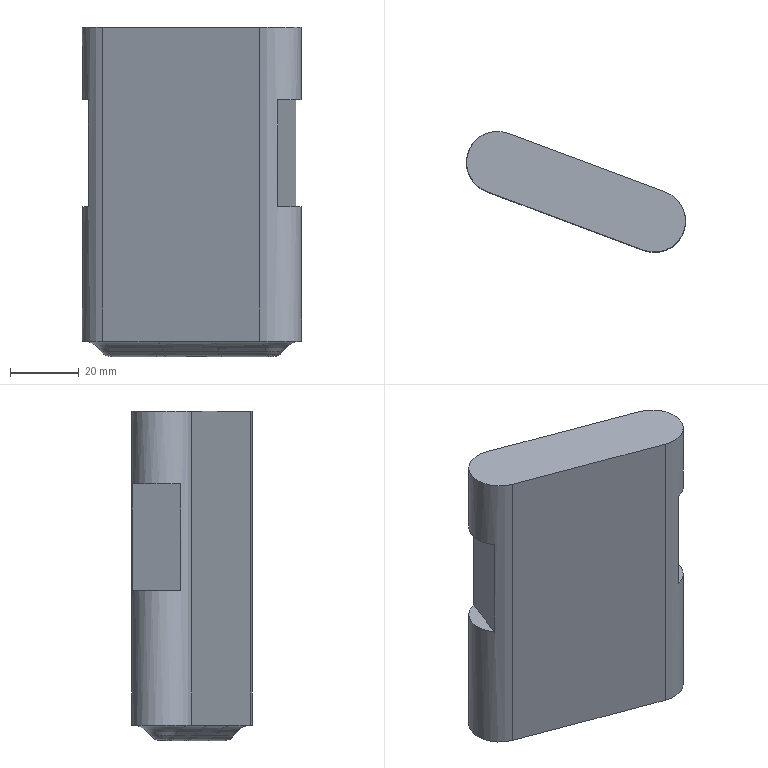Part | NX | features 8 2 | 1 solid | 31 faces | box 63.572 x 35.039 x 95.5 mm | volume 102490 mm3 | plane 11 | cylinder 10 | spline 8 | torus 2 | commonest cylinder face diameters 6 x4 13 x4 18 x2
STEP:
#1=CARTESIAN_POINT('',(108.541,59.531,91.));
#2=VERTEX_POINT('',#1);
#3=CARTESIAN_POINT('',(114.844,76.391,91.));
#4=VERTEX_POINT('',#3);
#5=CARTESIAN_POINT('',(111.693,67.961,91.));
#6=DIRECTION('',(0.,0.,-1.));
#7=DIRECTION('',(1.,0.,0.));
#8=AXIS2_PLACEMENT_3D('',#5,#6,#7);
#9=CIRCLE('',#8,9.);
#10=EDGE_CURVE('',#2,#4,#9,.T.);
#11=ORIENTED_EDGE('',*,*,#10,.F.);
#12=CARTESIAN_POINT('',(154.113,42.492,91.));
#13=VERTEX_POINT('',#12);
#14=CARTESIAN_POINT('',(154.113,42.492,91.));
#15=DIRECTION('',(0.9367,-0.3502,0.));
#16=VECTOR('',#15,1000.);
#17=LINE('',#14,#16);
#18=EDGE_CURVE('',#2,#13,#17,.T.);
#19=ORIENTED_EDGE('',*,*,#18,.T.);
#20=CARTESIAN_POINT('',(160.417,59.352,91.));
#21=VERTEX_POINT('',#20);
#22=CARTESIAN_POINT('',(157.265,50.922,91.));
#23=DIRECTION('',(0.,0.,-1.));
#24=DIRECTION('',(1.,0.,0.));
#25=AXIS2_PLACEMENT_3D('',#22,#23,#24);
#26=CIRCLE('',#25,9.);
#27=EDGE_CURVE('',#21,#13,#26,.T.);
#28=ORIENTED_EDGE('',*,*,#27,.F.);
#29=CARTESIAN_POINT('',(160.417,59.352,91.));
#30=DIRECTION('',(-0.9367,0.3502,0.));
#31=VECTOR('',#30,1000.);
#32=LINE('',#29,#31);
#33=EDGE_CURVE('',#21,#4,#32,.T.);
#34=ORIENTED_EDGE('',*,*,#33,.T.);
#35=EDGE_LOOP('',(#11,#19,#28,#34));
#36=FACE_BOUND('',#35,.T.);
#37=CARTESIAN_POINT('',(1075.,0.,91.));
#38=DIRECTION('',(0.,0.,1.));
#39=DIRECTION('',(-1.,0.,0.));
#40=AXIS2_PLACEMENT_3D('',#37,#38,#39);
#41=PLANE('',#40);
#42=ADVANCED_FACE('',(#36),#41,.T.);
#43=ORIENTED_EDGE('',*,*,#33,.F.);
#44=CARTESIAN_POINT('',(160.417,59.352,-0.0004651));
#45=VERTEX_POINT('',#44);
#46=CARTESIAN_POINT('',(160.417,59.352,-100.));
#47=DIRECTION('',(0.,0.,-1.));
#48=VECTOR('',#47,1000.);
#49=LINE('',#46,#48);
#50=EDGE_CURVE('',#21,#45,#49,.T.);
#51=ORIENTED_EDGE('',*,*,#50,.T.);
#52=CARTESIAN_POINT('',(146.714,64.517,-0.0002356));
#53=VERTEX_POINT('',#52);
#54=CARTESIAN_POINT('',(160.417,59.352,-0.0004651));
#55=CARTESIAN_POINT('',(156.358,60.87,-0.0004651));
#56=CARTESIAN_POINT('',(152.299,62.387,-0.0004651));
#57=CARTESIAN_POINT('',(147.727,64.097,-0.0004651));
#58=CARTESIAN_POINT('',(147.214,64.289,-0.0004651));
#59=CARTESIAN_POINT('',(146.7,64.48,-0.0004651));
#60=B_SPLINE_CURVE_WITH_KNOTS('',3,(#54,#55,#56,#57,#58,#59),.UNSPECIFIED.,.F.,.F.,(4,2,4),(0.,0.8877,1.),.UNSPECIFIED.);
#61=EDGE_CURVE('',#45,#53,#60,.T.);
#62=ORIENTED_EDGE('',*,*,#61,.T.);
#63=CARTESIAN_POINT('',(130.403,70.602,-0.0003097));
#64=VERTEX_POINT('',#63);
#65=CARTESIAN_POINT('',(130.393,70.577,-0.0004711));
#66=CARTESIAN_POINT('',(135.829,68.545,-0.0004711));
#67=CARTESIAN_POINT('',(141.265,66.513,-0.0004711));
#68=CARTESIAN_POINT('',(146.7,64.48,-0.0004711));
#69=B_SPLINE_CURVE_WITH_KNOTS('',3,(#65,#66,#67,#68),.UNSPECIFIED.,.F.,.F.,(4,4),(0.,1.),.PIECEWISE_BEZIER_KNOTS.);
#70=EDGE_CURVE('',#64,#53,#69,.T.);
#71=ORIENTED_EDGE('',*,*,#70,.F.);
#72=CARTESIAN_POINT('',(114.844,76.391,-0.0004651));
#73=VERTEX_POINT('',#72);
#74=CARTESIAN_POINT('',(130.393,70.577,-0.0004651));
#75=CARTESIAN_POINT('',(126.432,72.058,-0.0004651));
#76=CARTESIAN_POINT('',(122.471,73.539,-0.0004651));
#77=CARTESIAN_POINT('',(117.288,75.477,-0.0004651));
#78=CARTESIAN_POINT('',(116.066,75.934,-0.0004651));
#79=CARTESIAN_POINT('',(114.844,76.391,-0.0004651));
#80=B_SPLINE_CURVE_WITH_KNOTS('',3,(#74,#75,#76,#77,#78,#79),.UNSPECIFIED.,.F.,.F.,(4,2,4),(0.,0.7642,1.),.UNSPECIFIED.);
#81=EDGE_CURVE('',#64,#73,#80,.T.);
#82=ORIENTED_EDGE('',*,*,#81,.T.);
#83=CARTESIAN_POINT('',(114.844,76.391,-100.));
#84=DIRECTION('',(0.,0.,1.));
#85=VECTOR('',#84,1000.);
#86=LINE('',#83,#85);
#87=EDGE_CURVE('',#73,#4,#86,.T.);
#88=ORIENTED_EDGE('',*,*,#87,.T.);
#89=EDGE_LOOP('',(#43,#51,#62,#71,#82,#88));
#90=FACE_BOUND('',#89,.T.);
#91=CARTESIAN_POINT('',(160.417,59.352,-100.));
#92=DIRECTION('',(-0.3502,-0.9367,0.));
#93=DIRECTION('',(0.9367,-0.3502,0.));
#94=AXIS2_PLACEMENT_3D('',#91,#92,#93);
#95=PLANE('',#94);
#96=ADVANCED_FACE('',(#90),#95,.F.);
#97=CARTESIAN_POINT('',(159.328,42.162,70.));
#98=VERTEX_POINT('',#97);
#99=CARTESIAN_POINT('',(164.569,56.181,70.));
#100=VERTEX_POINT('',#99);
#101=CARTESIAN_POINT('',(157.265,50.922,70.));
#102=DIRECTION('',(0.,0.,1.));
#103=DIRECTION('',(1.,0.,0.));
#104=AXIS2_PLACEMENT_3D('',#101,#102,#103);
#105=CIRCLE('',#104,9.);
#106=EDGE_CURVE('',#98,#100,#105,.T.);
#107=ORIENTED_EDGE('',*,*,#106,.T.);
#108=CARTESIAN_POINT('',(164.569,56.181,39.));
#109=VERTEX_POINT('',#108);
#110=CARTESIAN_POINT('',(164.569,56.181,-100.));
#111=DIRECTION('',(0.,0.,-1.));
#112=VECTOR('',#111,1000.);
#113=LINE('',#110,#112);
#114=EDGE_CURVE('',#100,#109,#113,.T.);
#115=ORIENTED_EDGE('',*,*,#114,.T.);
#116=CARTESIAN_POINT('',(159.328,42.162,39.));
#117=VERTEX_POINT('',#116);
#118=CARTESIAN_POINT('',(157.265,50.922,39.));
#119=DIRECTION('',(0.,0.,-1.));
#120=DIRECTION('',(-1.,0.,0.));
#121=AXIS2_PLACEMENT_3D('',#118,#119,#120);
#122=CIRCLE('',#121,9.);
#123=EDGE_CURVE('',#109,#117,#122,.T.);
#124=ORIENTED_EDGE('',*,*,#123,.T.);
#125=CARTESIAN_POINT('',(159.328,42.162,-100.));
#126=DIRECTION('',(0.,0.,1.));
#127=VECTOR('',#126,1000.);
#128=LINE('',#125,#127);
#129=EDGE_CURVE('',#117,#98,#128,.T.);
#130=ORIENTED_EDGE('',*,*,#129,.T.);
#131=EDGE_LOOP('',(#107,#115,#124,#130));
#132=FACE_BOUND('',#131,.T.);
#133=ORIENTED_EDGE('',*,*,#27,.T.);
#134=CARTESIAN_POINT('',(154.113,42.492,-0.000465));
#135=VERTEX_POINT('',#134);
#136=CARTESIAN_POINT('',(154.113,42.492,-100.));
#137=DIRECTION('',(0.,0.,1.));
#138=VECTOR('',#137,1000.);
#139=LINE('',#136,#138);
#140=EDGE_CURVE('',#135,#13,#139,.T.);
#141=ORIENTED_EDGE('',*,*,#140,.F.);
#142=CARTESIAN_POINT('',(157.265,50.922,-0.000465));
#143=DIRECTION('',(-0.000000001,0.000000001,1.));
#144=DIRECTION('',(0.,-1.,0.000000001));
#145=AXIS2_PLACEMENT_3D('',#142,#143,#144);
#146=CIRCLE('',#145,9.);
#147=EDGE_CURVE('',#45,#135,#146,.F.);
#148=ORIENTED_EDGE('',*,*,#147,.F.);
#149=ORIENTED_EDGE('',*,*,#50,.F.);
#150=EDGE_LOOP('',(#133,#141,#148,#149));
#151=FACE_BOUND('',#150,.T.);
#152=CARTESIAN_POINT('',(157.265,50.922,-100.));
#153=DIRECTION('',(0.,0.,1.));
#154=DIRECTION('',(-1.,0.,0.));
#155=AXIS2_PLACEMENT_3D('',#152,#153,#154);
#156=CYLINDRICAL_SURFACE('',#155,9.);
#157=ADVANCED_FACE('',(#132,#151),#156,.T.);
#158=CARTESIAN_POINT('',(104.389,62.702,39.));
#159=VERTEX_POINT('',#158);
#160=CARTESIAN_POINT('',(109.63,76.721,39.));
#161=VERTEX_POINT('',#160);
#162=CARTESIAN_POINT('',(111.693,67.961,39.));
#163=DIRECTION('',(0.,0.,-1.));
#164=DIRECTION('',(-1.,0.,0.));
#165=AXIS2_PLACEMENT_3D('',#162,#163,#164);
#166=CIRCLE('',#165,9.);
#167=EDGE_CURVE('',#159,#161,#166,.T.);
#168=ORIENTED_EDGE('',*,*,#167,.T.);
#169=CARTESIAN_POINT('',(109.63,76.721,70.));
#170=VERTEX_POINT('',#169);
#171=CARTESIAN_POINT('',(109.63,76.721,-100.));
#172=DIRECTION('',(0.,0.,1.));
#173=VECTOR('',#172,1000.);
#174=LINE('',#171,#173);
#175=EDGE_CURVE('',#161,#170,#174,.T.);
#176=ORIENTED_EDGE('',*,*,#175,.T.);
#177=CARTESIAN_POINT('',(104.389,62.702,70.));
#178=VERTEX_POINT('',#177);
#179=CARTESIAN_POINT('',(111.693,67.961,70.));
#180=DIRECTION('',(0.,0.,1.));
#181=DIRECTION('',(1.,0.,0.));
#182=AXIS2_PLACEMENT_3D('',#179,#180,#181);
#183=CIRCLE('',#182,9.);
#184=EDGE_CURVE('',#170,#178,#183,.T.);
#185=ORIENTED_EDGE('',*,*,#184,.T.);
#186=CARTESIAN_POINT('',(104.389,62.702,-100.));
#187=DIRECTION('',(0.,0.,-1.));
#188=VECTOR('',#187,1000.);
#189=LINE('',#186,#188);
#190=EDGE_CURVE('',#178,#159,#189,.T.);
#191=ORIENTED_EDGE('',*,*,#190,.T.);
#192=EDGE_LOOP('',(#168,#176,#185,#191));
#193=FACE_BOUND('',#192,.T.);
#194=ORIENTED_EDGE('',*,*,#87,.F.);
#195=CARTESIAN_POINT('',(108.541,59.531,-0.0004651));
#196=VERTEX_POINT('',#195);
#197=CARTESIAN_POINT('',(111.693,67.961,-0.0004651));
#198=DIRECTION('',(0.000000001,-0.000000001,-1.));
#199=DIRECTION('',(0.,1.,-0.000000001));
#200=AXIS2_PLACEMENT_3D('',#197,#198,#199);
#201=CIRCLE('',#200,9.);
#202=EDGE_CURVE('',#196,#73,#201,.T.);
#203=ORIENTED_EDGE('',*,*,#202,.F.);
#204=CARTESIAN_POINT('',(108.541,59.531,-100.));
#205=DIRECTION('',(0.,0.,-1.));
#206=VECTOR('',#205,1000.);
#207=LINE('',#204,#206);
#208=EDGE_CURVE('',#2,#196,#207,.T.);
#209=ORIENTED_EDGE('',*,*,#208,.F.);
#210=ORIENTED_EDGE('',*,*,#10,.T.);
#211=EDGE_LOOP('',(#194,#203,#209,#210));
#212=FACE_BOUND('',#211,.T.);
#213=CARTESIAN_POINT('',(111.693,67.961,-100.));
#214=DIRECTION('',(0.,0.,-1.));
#215=DIRECTION('',(1.,0.,0.));
#216=AXIS2_PLACEMENT_3D('',#213,#214,#215);
#217=CYLINDRICAL_SURFACE('',#216,9.);
#218=ADVANCED_FACE('',(#193,#212),#217,.T.);
#219=ORIENTED_EDGE('',*,*,#208,.T.);
#220=CARTESIAN_POINT('',(124.09,53.717,-0.0004681));
#221=VERTEX_POINT('',#220);
#222=CARTESIAN_POINT('',(108.541,59.531,-0.0004651));
#223=CARTESIAN_POINT('',(112.6,58.013,-0.0004651));
#224=CARTESIAN_POINT('',(116.658,56.496,-0.0004651));
#225=CARTESIAN_POINT('',(121.841,54.558,-0.0004651));
#226=CARTESIAN_POINT('',(122.966,54.137,-0.0004651));
#227=CARTESIAN_POINT('',(124.09,53.717,-0.0004651));
#228=B_SPLINE_CURVE_WITH_KNOTS('',3,(#222,#223,#224,#225,#226,#227),.UNSPECIFIED.,.F.,.F.,(4,2,4),(0.,0.7831,1.),.UNSPECIFIED.);
#229=EDGE_CURVE('',#196,#221,#228,.T.);
#230=ORIENTED_EDGE('',*,*,#229,.T.);
#231=CARTESIAN_POINT('',(140.397,47.62,-0.000468));
#232=VERTEX_POINT('',#231);
#233=CARTESIAN_POINT('',(140.397,47.62,-0.000471));
#234=CARTESIAN_POINT('',(134.961,49.653,-0.000471));
#235=CARTESIAN_POINT('',(129.525,51.685,-0.0004711));
#236=CARTESIAN_POINT('',(124.09,53.717,-0.0004711));
#237=B_SPLINE_CURVE_WITH_KNOTS('',3,(#233,#234,#235,#236),.UNSPECIFIED.,.F.,.F.,(4,4),(0.,1.),.PIECEWISE_BEZIER_KNOTS.);
#238=EDGE_CURVE('',#232,#221,#237,.T.);
#239=ORIENTED_EDGE('',*,*,#238,.F.);
#240=CARTESIAN_POINT('',(140.397,47.62,-0.0004651));
#241=CARTESIAN_POINT('',(144.445,46.107,-0.0004651));
#242=CARTESIAN_POINT('',(148.494,44.593,-0.000465));
#243=CARTESIAN_POINT('',(153.066,42.884,-0.000465));
#244=CARTESIAN_POINT('',(153.589,42.688,-0.000465));
#245=CARTESIAN_POINT('',(154.113,42.492,-0.000465));
#246=B_SPLINE_CURVE_WITH_KNOTS('',3,(#240,#241,#242,#243,#244,#245),.UNSPECIFIED.,.F.,.F.,(4,2,4),(0.,0.8855,1.),.UNSPECIFIED.);
#247=EDGE_CURVE('',#232,#135,#246,.T.);
#248=ORIENTED_EDGE('',*,*,#247,.T.);
#249=ORIENTED_EDGE('',*,*,#140,.T.);
#250=ORIENTED_EDGE('',*,*,#18,.F.);
#251=EDGE_LOOP('',(#219,#230,#239,#248,#249,#250));
#252=FACE_BOUND('',#251,.T.);
#253=CARTESIAN_POINT('',(154.113,42.492,-100.));
#254=DIRECTION('',(0.3502,0.9367,0.));
#255=DIRECTION('',(0.9367,-0.3502,0.));
#256=AXIS2_PLACEMENT_3D('',#253,#254,#255);
#257=PLANE('',#256);
#258=ADVANCED_FACE('',(#252),#257,.F.);
#259=CARTESIAN_POINT('',(143.899,56.987,-4.5));
#260=VERTEX_POINT('',#259);
#261=CARTESIAN_POINT('',(157.615,51.859,-4.5));
#262=VERTEX_POINT('',#261);
#263=CARTESIAN_POINT('',(150.757,54.423,-4.5));
#264=DIRECTION('',(0.9367,-0.3502,0.000000001));
#265=VECTOR('',#264,1000.);
#266=LINE('',#263,#265);
#267=EDGE_CURVE('',#260,#262,#266,.T.);
#268=ORIENTED_EDGE('',*,*,#267,.T.);
#269=CARTESIAN_POINT('',(156.915,49.985,-4.5));
#270=VERTEX_POINT('',#269);
#271=CARTESIAN_POINT('',(157.265,50.922,-4.5));
#272=DIRECTION('',(-0.000000001,0.000000001,1.));
#273=DIRECTION('',(-0.09584,-0.9954,0.000000001));
#274=AXIS2_PLACEMENT_3D('',#271,#272,#273);
#275=CIRCLE('',#274,1.);
#276=EDGE_CURVE('',#270,#262,#275,.T.);
#277=ORIENTED_EDGE('',*,*,#276,.F.);
#278=CARTESIAN_POINT('',(143.198,55.114,-4.5));
#279=VERTEX_POINT('',#278);
#280=CARTESIAN_POINT('',(150.057,52.55,-4.5));
#281=DIRECTION('',(0.9367,-0.3502,0.000000001));
#282=VECTOR('',#281,1000.);
#283=LINE('',#280,#282);
#284=EDGE_CURVE('',#279,#270,#283,.T.);
#285=ORIENTED_EDGE('',*,*,#284,.F.);
#286=CARTESIAN_POINT('',(126.891,61.211,-4.5));
#287=VERTEX_POINT('',#286);
#288=CARTESIAN_POINT('',(126.891,61.211,-4.5));
#289=CARTESIAN_POINT('',(132.327,59.178,-4.5));
#290=CARTESIAN_POINT('',(137.763,57.146,-4.5));
#291=CARTESIAN_POINT('',(143.198,55.114,-4.5));
#292=B_SPLINE_CURVE_WITH_KNOTS('',3,(#288,#289,#290,#291),.UNSPECIFIED.,.F.,.F.,(4,4),(0.,1.),.PIECEWISE_BEZIER_KNOTS.);
#293=EDGE_CURVE('',#287,#279,#292,.T.);
#294=ORIENTED_EDGE('',*,*,#293,.F.);
#295=CARTESIAN_POINT('',(124.472,62.115,-4.5));
#296=VERTEX_POINT('',#295);
#297=CARTESIAN_POINT('',(125.681,61.663,-4.5));
#298=DIRECTION('',(0.9367,-0.3502,0.000000001));
#299=VECTOR('',#298,1000.);
#300=LINE('',#297,#299);
#301=EDGE_CURVE('',#296,#287,#300,.T.);
#302=ORIENTED_EDGE('',*,*,#301,.F.);
#303=CARTESIAN_POINT('',(125.172,63.989,-4.5));
#304=VERTEX_POINT('',#303);
#305=CARTESIAN_POINT('',(125.172,63.989,-4.5));
#306=CARTESIAN_POINT('',(124.472,62.115,-4.5));
#307=B_SPLINE_CURVE_WITH_KNOTS('',1,(#305,#306),.UNSPECIFIED.,.F.,.F.,(2,2),(0.,1.),.PIECEWISE_BEZIER_KNOTS.);
#308=EDGE_CURVE('',#304,#296,#307,.T.);
#309=ORIENTED_EDGE('',*,*,#308,.F.);
#310=CARTESIAN_POINT('',(127.592,63.084,-4.5));
#311=VERTEX_POINT('',#310);
#312=CARTESIAN_POINT('',(126.382,63.536,-4.5));
#313=DIRECTION('',(-0.9367,0.3502,-0.000000001));
#314=VECTOR('',#313,1000.);
#315=LINE('',#312,#314);
#316=EDGE_CURVE('',#311,#304,#315,.T.);
#317=ORIENTED_EDGE('',*,*,#316,.F.);
#318=CARTESIAN_POINT('',(127.592,63.084,-4.5));
#319=CARTESIAN_POINT('',(133.027,61.052,-4.5));
#320=CARTESIAN_POINT('',(138.463,59.019,-4.5));
#321=CARTESIAN_POINT('',(143.899,56.987,-4.5));
#322=B_SPLINE_CURVE_WITH_KNOTS('',3,(#318,#319,#320,#321),.UNSPECIFIED.,.F.,.F.,(4,4),(0.,1.),.PIECEWISE_BEZIER_KNOTS.);
#323=EDGE_CURVE('',#311,#260,#322,.T.);
#324=ORIENTED_EDGE('',*,*,#323,.T.);
#325=EDGE_LOOP('',(#268,#277,#285,#294,#302,#309,#317,#324));
#326=FACE_BOUND('',#325,.T.);
#327=CARTESIAN_POINT('',(143.198,55.114,-4.5));
#328=DIRECTION('',(-0.000000001,0.000000001,1.));
#329=DIRECTION('',(-0.9367,0.3502,-0.000000001));
#330=AXIS2_PLACEMENT_3D('',#327,#328,#329);
#331=PLANE('',#330);
#332=ADVANCED_FACE('',(#326),#331,.F.);
#333=ORIENTED_EDGE('',*,*,#308,.T.);
#334=CARTESIAN_POINT('',(111.342,67.024,-4.5));
#335=VERTEX_POINT('',#334);
#336=CARTESIAN_POINT('',(111.342,67.024,-4.5));
#337=CARTESIAN_POINT('',(115.719,65.388,-4.5));
#338=CARTESIAN_POINT('',(120.095,63.751,-4.5));
#339=CARTESIAN_POINT('',(124.472,62.115,-4.5));
#340=B_SPLINE_CURVE_WITH_KNOTS('',3,(#336,#337,#338,#339),.UNSPECIFIED.,.F.,.F.,(4,4),(0.,1.),.PIECEWISE_BEZIER_KNOTS.);
#341=EDGE_CURVE('',#335,#296,#340,.T.);
#342=ORIENTED_EDGE('',*,*,#341,.F.);
#343=CARTESIAN_POINT('',(112.043,68.897,-4.5));
#344=VERTEX_POINT('',#343);
#345=CARTESIAN_POINT('',(112.043,68.897,-4.5));
#346=CARTESIAN_POINT('',(111.552,69.081,-4.5));
#347=CARTESIAN_POINT('',(110.939,68.801,-4.5));
#348=CARTESIAN_POINT('',(110.573,67.82,-4.5));
#349=CARTESIAN_POINT('',(110.852,67.207,-4.5));
#350=CARTESIAN_POINT('',(111.342,67.024,-4.5));
#351=B_SPLINE_CURVE_WITH_KNOTS('',3,(#345,#346,#347,#348,#349,#350),.UNSPECIFIED.,.F.,.F.,(4,2,4),(0.,0.5,1.),.UNSPECIFIED.);
#352=EDGE_CURVE('',#344,#335,#351,.T.);
#353=ORIENTED_EDGE('',*,*,#352,.F.);
#354=CARTESIAN_POINT('',(112.043,68.897,-4.5));
#355=CARTESIAN_POINT('',(125.172,63.989,-4.5));
#356=B_SPLINE_CURVE_WITH_KNOTS('',1,(#354,#355),.UNSPECIFIED.,.F.,.F.,(2,2),(0.,1.),.PIECEWISE_BEZIER_KNOTS.);
#357=EDGE_CURVE('',#344,#304,#356,.T.);
#358=ORIENTED_EDGE('',*,*,#357,.T.);
#359=EDGE_LOOP('',(#333,#342,#353,#358));
#360=FACE_BOUND('',#359,.T.);
#361=CARTESIAN_POINT('',(126.891,61.211,-4.5));
#362=DIRECTION('',(0.000000001,-0.000000001,-1.));
#363=DIRECTION('',(0.9367,-0.3502,0.000000001));
#364=AXIS2_PLACEMENT_3D('',#361,#362,#363);
#365=PLANE('',#364);
#366=ADVANCED_FACE('',(#360),#365,.T.);
#367=CARTESIAN_POINT('',(126.065,66.378,-3.079));
#368=VERTEX_POINT('',#367);
#369=CARTESIAN_POINT('',(128.485,65.473,-3.079));
#370=VERTEX_POINT('',#369);
#371=CARTESIAN_POINT('',(127.275,65.926,-3.079));
#372=DIRECTION('',(0.9367,-0.3502,0.000000001));
#373=VECTOR('',#372,1000.);
#374=LINE('',#371,#373);
#375=EDGE_CURVE('',#368,#370,#374,.T.);
#376=ORIENTED_EDGE('',*,*,#375,.T.);
#377=CARTESIAN_POINT('',(128.485,65.473,-3.079));
#378=CARTESIAN_POINT('',(128.298,64.972,-3.943));
#379=CARTESIAN_POINT('',(127.948,64.036,-4.5));
#380=CARTESIAN_POINT('',(127.592,63.084,-4.5));
#381=B_SPLINE_CURVE_WITH_KNOTS('',3,(#377,#378,#379,#380),.UNSPECIFIED.,.F.,.F.,(4,4),(0.,1.),.UNSPECIFIED.);
#382=EDGE_CURVE('',#370,#311,#381,.T.);
#383=ORIENTED_EDGE('',*,*,#382,.T.);
#384=ORIENTED_EDGE('',*,*,#316,.T.);
#385=CARTESIAN_POINT('',(125.172,63.989,-4.5));
#386=CARTESIAN_POINT('',(125.528,64.941,-4.5));
#387=CARTESIAN_POINT('',(125.878,65.877,-3.943));
#388=CARTESIAN_POINT('',(126.065,66.378,-3.079));
#389=B_SPLINE_CURVE_WITH_KNOTS('',3,(#385,#386,#387,#388),.UNSPECIFIED.,.F.,.F.,(4,4),(0.,1.),.UNSPECIFIED.);
#390=EDGE_CURVE('',#368,#304,#389,.F.);
#391=ORIENTED_EDGE('',*,*,#390,.F.);
#392=EDGE_LOOP('',(#376,#383,#384,#391));
#393=FACE_BOUND('',#392,.T.);
#394=CARTESIAN_POINT('',(136.129,59.892,-1.5));
#395=DIRECTION('',(0.9367,-0.3502,0.000000001));
#396=DIRECTION('',(-0.000000001,0.000000001,1.));
#397=AXIS2_PLACEMENT_3D('',#394,#395,#396);
#398=CYLINDRICAL_SURFACE('',#397,3.);
#399=ADVANCED_FACE('',(#393),#398,.T.);
#400=CARTESIAN_POINT('',(112.936,71.287,-3.079));
#401=VERTEX_POINT('',#400);
#402=CARTESIAN_POINT('',(112.043,68.897,-4.5));
#403=CARTESIAN_POINT('',(112.384,69.809,-4.5));
#404=CARTESIAN_POINT('',(112.757,70.807,-3.907));
#405=CARTESIAN_POINT('',(112.936,71.287,-3.079));
#406=B_SPLINE_CURVE_WITH_KNOTS('',3,(#402,#403,#404,#405),.UNSPECIFIED.,.F.,.F.,(4,4),(0.,1.),.UNSPECIFIED.);
#407=EDGE_CURVE('',#401,#344,#406,.F.);
#408=ORIENTED_EDGE('',*,*,#407,.F.);
#409=CARTESIAN_POINT('',(112.936,71.287,-3.079));
#410=CARTESIAN_POINT('',(117.312,69.65,-3.079));
#411=CARTESIAN_POINT('',(121.689,68.014,-3.079));
#412=CARTESIAN_POINT('',(126.065,66.378,-3.079));
#413=B_SPLINE_CURVE_WITH_KNOTS('',3,(#409,#410,#411,#412),.UNSPECIFIED.,.F.,.F.,(4,4),(0.,1.),.PIECEWISE_BEZIER_KNOTS.);
#414=EDGE_CURVE('',#401,#368,#413,.T.);
#415=ORIENTED_EDGE('',*,*,#414,.T.);
#416=ORIENTED_EDGE('',*,*,#390,.T.);
#417=ORIENTED_EDGE('',*,*,#357,.F.);
#418=EDGE_LOOP('',(#408,#415,#416,#417));
#419=FACE_BOUND('',#418,.T.);
#420=CARTESIAN_POINT('',(112.043,68.897,-4.5));
#421=CARTESIAN_POINT('',(116.419,67.261,-4.5));
#422=CARTESIAN_POINT('',(120.796,65.625,-4.5));
#423=CARTESIAN_POINT('',(125.172,63.989,-4.5));
#424=CARTESIAN_POINT('',(112.128,69.125,-4.5));
#425=CARTESIAN_POINT('',(116.504,67.489,-4.5));
#426=CARTESIAN_POINT('',(120.881,65.853,-4.5));
#427=CARTESIAN_POINT('',(125.257,64.217,-4.5));
#428=CARTESIAN_POINT('',(112.304,69.596,-4.44));
#429=CARTESIAN_POINT('',(116.68,67.96,-4.44));
#430=CARTESIAN_POINT('',(121.057,66.324,-4.44));
#431=CARTESIAN_POINT('',(125.433,64.687,-4.44));
#432=CARTESIAN_POINT('',(112.56,70.28,-4.151));
#433=CARTESIAN_POINT('',(116.936,68.644,-4.151));
#434=CARTESIAN_POINT('',(121.313,67.008,-4.151));
#435=CARTESIAN_POINT('',(125.689,65.372,-4.151));
#436=CARTESIAN_POINT('',(112.781,70.871,-3.682));
#437=CARTESIAN_POINT('',(117.157,69.235,-3.682));
#438=CARTESIAN_POINT('',(121.533,67.599,-3.682));
#439=CARTESIAN_POINT('',(125.91,65.962,-3.682));
#440=CARTESIAN_POINT('',(112.891,71.167,-3.286));
#441=CARTESIAN_POINT('',(117.268,69.53,-3.286));
#442=CARTESIAN_POINT('',(121.644,67.894,-3.286));
#443=CARTESIAN_POINT('',(126.02,66.258,-3.286));
#444=CARTESIAN_POINT('',(112.936,71.287,-3.079));
#445=CARTESIAN_POINT('',(117.312,69.65,-3.079));
#446=CARTESIAN_POINT('',(121.689,68.014,-3.079));
#447=CARTESIAN_POINT('',(126.065,66.378,-3.079));
#448=B_SPLINE_SURFACE_WITH_KNOTS('',3,3,((#420,#421,#422,#423),(#424,#425,#426,#427),(#428,#429,#430,#431),(#432,#433,#434,#435),(#436,#437,#438,#439),(#440,#441,#442,#443),(#444,#445,#446,#447)),.SURF_OF_LINEAR_EXTRUSION.,.F.,.F.,.F.,(4,1,1,1,4),(4,4),(0.,0.25,0.5,0.75,1.),(0.,1.),.UNSPECIFIED.);
#449=ADVANCED_FACE('',(#419),#448,.T.);
#450=CARTESIAN_POINT('',(144.792,59.376,-3.079));
#451=VERTEX_POINT('',#450);
#452=CARTESIAN_POINT('',(158.508,54.248,-3.079));
#453=VERTEX_POINT('',#452);
#454=CARTESIAN_POINT('',(151.65,56.812,-3.079));
#455=DIRECTION('',(0.9367,-0.3502,0.000000001));
#456=VECTOR('',#455,1000.);
#457=LINE('',#454,#456);
#458=EDGE_CURVE('',#451,#453,#457,.T.);
#459=ORIENTED_EDGE('',*,*,#458,.T.);
#460=CARTESIAN_POINT('',(157.615,51.859,-1.5));
#461=DIRECTION('',(0.9367,-0.3502,0.000000001));
#462=DIRECTION('',(-0.3502,-0.9367,0.000000001));
#463=AXIS2_PLACEMENT_3D('',#460,#461,#462);
#464=CIRCLE('',#463,3.);
#465=EDGE_CURVE('',#262,#453,#464,.T.);
#466=ORIENTED_EDGE('',*,*,#465,.F.);
#467=ORIENTED_EDGE('',*,*,#267,.F.);
#468=CARTESIAN_POINT('',(143.899,56.987,-4.5));
#469=CARTESIAN_POINT('',(144.255,57.939,-4.5));
#470=CARTESIAN_POINT('',(144.605,58.875,-3.943));
#471=CARTESIAN_POINT('',(144.792,59.376,-3.079));
#472=B_SPLINE_CURVE_WITH_KNOTS('',3,(#468,#469,#470,#471),.UNSPECIFIED.,.F.,.F.,(4,4),(0.,1.),.UNSPECIFIED.);
#473=EDGE_CURVE('',#260,#451,#472,.T.);
#474=ORIENTED_EDGE('',*,*,#473,.T.);
#475=EDGE_LOOP('',(#459,#466,#467,#474));
#476=FACE_BOUND('',#475,.T.);
#477=CARTESIAN_POINT('',(135.603,60.089,-1.5));
#478=DIRECTION('',(-0.9367,0.3502,-0.000000001));
#479=DIRECTION('',(-0.2978,-0.7964,0.5263));
#480=AXIS2_PLACEMENT_3D('',#477,#478,#479);
#481=CYLINDRICAL_SURFACE('',#480,3.);
#482=ADVANCED_FACE('',(#476),#481,.T.);
#483=ORIENTED_EDGE('',*,*,#382,.F.);
#484=CARTESIAN_POINT('',(128.485,65.473,-3.079));
#485=CARTESIAN_POINT('',(133.921,63.441,-3.079));
#486=CARTESIAN_POINT('',(139.356,61.409,-3.079));
#487=CARTESIAN_POINT('',(144.792,59.376,-3.079));
#488=B_SPLINE_CURVE_WITH_KNOTS('',3,(#484,#485,#486,#487),.UNSPECIFIED.,.F.,.F.,(4,4),(0.,1.),.PIECEWISE_BEZIER_KNOTS.);
#489=EDGE_CURVE('',#370,#451,#488,.T.);
#490=ORIENTED_EDGE('',*,*,#489,.T.);
#491=ORIENTED_EDGE('',*,*,#473,.F.);
#492=ORIENTED_EDGE('',*,*,#323,.F.);
#493=EDGE_LOOP('',(#483,#490,#491,#492));
#494=FACE_BOUND('',#493,.T.);
#495=CARTESIAN_POINT('',(127.592,63.084,-4.5));
#496=CARTESIAN_POINT('',(133.027,61.052,-4.5));
#497=CARTESIAN_POINT('',(138.463,59.019,-4.5));
#498=CARTESIAN_POINT('',(143.899,56.987,-4.5));
#499=CARTESIAN_POINT('',(127.677,63.312,-4.5));
#500=CARTESIAN_POINT('',(133.113,61.28,-4.5));
#501=CARTESIAN_POINT('',(138.548,59.247,-4.5));
#502=CARTESIAN_POINT('',(143.984,57.215,-4.5));
#503=CARTESIAN_POINT('',(127.853,63.783,-4.44));
#504=CARTESIAN_POINT('',(133.289,61.75,-4.44));
#505=CARTESIAN_POINT('',(138.724,59.718,-4.44));
#506=CARTESIAN_POINT('',(144.16,57.686,-4.44));
#507=CARTESIAN_POINT('',(128.109,64.467,-4.151));
#508=CARTESIAN_POINT('',(133.545,62.435,-4.151));
#509=CARTESIAN_POINT('',(138.98,60.402,-4.151));
#510=CARTESIAN_POINT('',(144.416,58.37,-4.151));
#511=CARTESIAN_POINT('',(128.33,65.058,-3.682));
#512=CARTESIAN_POINT('',(133.765,63.025,-3.682));
#513=CARTESIAN_POINT('',(139.201,60.993,-3.682));
#514=CARTESIAN_POINT('',(144.637,58.961,-3.682));
#515=CARTESIAN_POINT('',(128.44,65.353,-3.286));
#516=CARTESIAN_POINT('',(133.876,63.321,-3.286));
#517=CARTESIAN_POINT('',(139.312,61.289,-3.286));
#518=CARTESIAN_POINT('',(144.747,59.256,-3.286));
#519=CARTESIAN_POINT('',(128.485,65.473,-3.079));
#520=CARTESIAN_POINT('',(133.921,63.441,-3.079));
#521=CARTESIAN_POINT('',(139.356,61.409,-3.079));
#522=CARTESIAN_POINT('',(144.792,59.376,-3.079));
#523=B_SPLINE_SURFACE_WITH_KNOTS('',3,3,((#495,#496,#497,#498),(#499,#500,#501,#502),(#503,#504,#505,#506),(#507,#508,#509,#510),(#511,#512,#513,#514),(#515,#516,#517,#518),(#519,#520,#521,#522)),.SURF_OF_LINEAR_EXTRUSION.,.F.,.F.,.F.,(4,1,1,1,4),(4,4),(0.,0.25,0.5,0.75,1.),(0.,1.),.UNSPECIFIED.);
#524=ADVANCED_FACE('',(#494),#523,.T.);
#525=CARTESIAN_POINT('',(125.998,58.821,-3.079));
#526=VERTEX_POINT('',#525);
#527=CARTESIAN_POINT('',(126.891,61.211,-4.5));
#528=CARTESIAN_POINT('',(126.535,60.258,-4.5));
#529=CARTESIAN_POINT('',(126.185,59.322,-3.943));
#530=CARTESIAN_POINT('',(125.998,58.821,-3.079));
#531=B_SPLINE_CURVE_WITH_KNOTS('',3,(#527,#528,#529,#530),.UNSPECIFIED.,.F.,.F.,(4,4),(0.,1.),.UNSPECIFIED.);
#532=EDGE_CURVE('',#287,#526,#531,.T.);
#533=ORIENTED_EDGE('',*,*,#532,.F.);
#534=ORIENTED_EDGE('',*,*,#293,.T.);
#535=CARTESIAN_POINT('',(142.305,52.724,-3.079));
#536=VERTEX_POINT('',#535);
#537=CARTESIAN_POINT('',(142.305,52.724,-3.079));
#538=CARTESIAN_POINT('',(142.492,53.225,-3.943));
#539=CARTESIAN_POINT('',(142.842,54.161,-4.5));
#540=CARTESIAN_POINT('',(143.198,55.114,-4.5));
#541=B_SPLINE_CURVE_WITH_KNOTS('',3,(#537,#538,#539,#540),.UNSPECIFIED.,.F.,.F.,(4,4),(0.,1.),.UNSPECIFIED.);
#542=EDGE_CURVE('',#279,#536,#541,.F.);
#543=ORIENTED_EDGE('',*,*,#542,.T.);
#544=CARTESIAN_POINT('',(125.998,58.821,-3.079));
#545=CARTESIAN_POINT('',(131.434,56.789,-3.079));
#546=CARTESIAN_POINT('',(136.869,54.757,-3.079));
#547=CARTESIAN_POINT('',(142.305,52.724,-3.079));
#548=B_SPLINE_CURVE_WITH_KNOTS('',3,(#544,#545,#546,#547),.UNSPECIFIED.,.F.,.F.,(4,4),(0.,1.),.PIECEWISE_BEZIER_KNOTS.);
#549=EDGE_CURVE('',#526,#536,#548,.T.);
#550=ORIENTED_EDGE('',*,*,#549,.F.);
#551=EDGE_LOOP('',(#533,#534,#543,#550));
#552=FACE_BOUND('',#551,.T.);
#553=CARTESIAN_POINT('',(125.998,58.821,-3.079));
#554=CARTESIAN_POINT('',(131.434,56.789,-3.079));
#555=CARTESIAN_POINT('',(136.869,54.757,-3.079));
#556=CARTESIAN_POINT('',(142.305,52.724,-3.079));
#557=CARTESIAN_POINT('',(126.043,58.941,-3.286));
#558=CARTESIAN_POINT('',(131.478,56.909,-3.286));
#559=CARTESIAN_POINT('',(136.914,54.877,-3.286));
#560=CARTESIAN_POINT('',(142.35,52.844,-3.286));
#561=CARTESIAN_POINT('',(126.153,59.237,-3.682));
#562=CARTESIAN_POINT('',(131.589,57.205,-3.682));
#563=CARTESIAN_POINT('',(137.025,55.172,-3.682));
#564=CARTESIAN_POINT('',(142.46,53.14,-3.682));
#565=CARTESIAN_POINT('',(126.374,59.827,-4.151));
#566=CARTESIAN_POINT('',(131.81,57.795,-4.151));
#567=CARTESIAN_POINT('',(137.246,55.763,-4.151));
#568=CARTESIAN_POINT('',(142.681,53.73,-4.151));
#569=CARTESIAN_POINT('',(126.63,60.512,-4.44));
#570=CARTESIAN_POINT('',(132.066,58.479,-4.44));
#571=CARTESIAN_POINT('',(137.501,56.447,-4.44));
#572=CARTESIAN_POINT('',(142.937,54.415,-4.44));
#573=CARTESIAN_POINT('',(126.806,60.983,-4.5));
#574=CARTESIAN_POINT('',(132.242,58.95,-4.5));
#575=CARTESIAN_POINT('',(137.677,56.918,-4.5));
#576=CARTESIAN_POINT('',(143.113,54.886,-4.5));
#577=CARTESIAN_POINT('',(126.891,61.211,-4.5));
#578=CARTESIAN_POINT('',(132.327,59.178,-4.5));
#579=CARTESIAN_POINT('',(137.763,57.146,-4.5));
#580=CARTESIAN_POINT('',(143.198,55.114,-4.5));
#581=B_SPLINE_SURFACE_WITH_KNOTS('',3,3,((#553,#554,#555,#556),(#557,#558,#559,#560),(#561,#562,#563,#564),(#565,#566,#567,#568),(#569,#570,#571,#572),(#573,#574,#575,#576),(#577,#578,#579,#580)),.SURF_OF_LINEAR_EXTRUSION.,.F.,.F.,.F.,(4,1,1,1,4),(4,4),(0.,0.25,0.5,0.75,1.),(0.,1.),.UNSPECIFIED.);
#582=ADVANCED_FACE('',(#552),#581,.T.);
#583=CARTESIAN_POINT('',(110.449,64.635,-3.079));
#584=VERTEX_POINT('',#583);
#585=CARTESIAN_POINT('',(110.449,64.635,-3.079));
#586=CARTESIAN_POINT('',(110.628,65.114,-3.907));
#587=CARTESIAN_POINT('',(111.001,66.112,-4.5));
#588=CARTESIAN_POINT('',(111.342,67.024,-4.5));
#589=B_SPLINE_CURVE_WITH_KNOTS('',3,(#585,#586,#587,#588),.UNSPECIFIED.,.F.,.F.,(4,4),(0.,1.),.UNSPECIFIED.);
#590=EDGE_CURVE('',#584,#335,#589,.T.);
#591=ORIENTED_EDGE('',*,*,#590,.T.);
#592=ORIENTED_EDGE('',*,*,#341,.T.);
#593=CARTESIAN_POINT('',(123.578,59.726,-3.079));
#594=VERTEX_POINT('',#593);
#595=CARTESIAN_POINT('',(123.578,59.726,-3.079));
#596=CARTESIAN_POINT('',(123.766,60.227,-3.943));
#597=CARTESIAN_POINT('',(124.116,61.163,-4.5));
#598=CARTESIAN_POINT('',(124.472,62.115,-4.5));
#599=B_SPLINE_CURVE_WITH_KNOTS('',3,(#595,#596,#597,#598),.UNSPECIFIED.,.F.,.F.,(4,4),(0.,1.),.UNSPECIFIED.);
#600=EDGE_CURVE('',#296,#594,#599,.F.);
#601=ORIENTED_EDGE('',*,*,#600,.T.);
#602=CARTESIAN_POINT('',(123.578,59.726,-3.079));
#603=CARTESIAN_POINT('',(119.202,61.362,-3.079));
#604=CARTESIAN_POINT('',(114.825,62.998,-3.079));
#605=CARTESIAN_POINT('',(110.449,64.635,-3.079));
#606=B_SPLINE_CURVE_WITH_KNOTS('',3,(#602,#603,#604,#605),.UNSPECIFIED.,.F.,.F.,(4,4),(0.,1.),.PIECEWISE_BEZIER_KNOTS.);
#607=EDGE_CURVE('',#594,#584,#606,.T.);
#608=ORIENTED_EDGE('',*,*,#607,.T.);
#609=EDGE_LOOP('',(#591,#592,#601,#608));
#610=FACE_BOUND('',#609,.T.);
#611=CARTESIAN_POINT('',(110.449,64.635,-3.079));
#612=CARTESIAN_POINT('',(114.825,62.998,-3.079));
#613=CARTESIAN_POINT('',(119.202,61.362,-3.079));
#614=CARTESIAN_POINT('',(123.578,59.726,-3.079));
#615=CARTESIAN_POINT('',(110.494,64.755,-3.286));
#616=CARTESIAN_POINT('',(114.87,63.118,-3.286));
#617=CARTESIAN_POINT('',(119.247,61.482,-3.286));
#618=CARTESIAN_POINT('',(123.623,59.846,-3.286));
#619=CARTESIAN_POINT('',(110.604,65.05,-3.682));
#620=CARTESIAN_POINT('',(114.981,63.414,-3.682));
#621=CARTESIAN_POINT('',(119.357,61.778,-3.682));
#622=CARTESIAN_POINT('',(123.734,60.142,-3.682));
#623=CARTESIAN_POINT('',(110.825,65.641,-4.151));
#624=CARTESIAN_POINT('',(115.202,64.005,-4.151));
#625=CARTESIAN_POINT('',(119.578,62.368,-4.151));
#626=CARTESIAN_POINT('',(123.954,60.732,-4.151));
#627=CARTESIAN_POINT('',(111.081,66.325,-4.44));
#628=CARTESIAN_POINT('',(115.457,64.689,-4.44));
#629=CARTESIAN_POINT('',(119.834,63.053,-4.44));
#630=CARTESIAN_POINT('',(124.21,61.416,-4.44));
#631=CARTESIAN_POINT('',(111.257,66.796,-4.5));
#632=CARTESIAN_POINT('',(115.634,65.16,-4.5));
#633=CARTESIAN_POINT('',(120.01,63.524,-4.5));
#634=CARTESIAN_POINT('',(124.386,61.887,-4.5));
#635=CARTESIAN_POINT('',(111.342,67.024,-4.5));
#636=CARTESIAN_POINT('',(115.719,65.388,-4.5));
#637=CARTESIAN_POINT('',(120.095,63.751,-4.5));
#638=CARTESIAN_POINT('',(124.472,62.115,-4.5));
#639=B_SPLINE_SURFACE_WITH_KNOTS('',3,3,((#611,#612,#613,#614),(#615,#616,#617,#618),(#619,#620,#621,#622),(#623,#624,#625,#626),(#627,#628,#629,#630),(#631,#632,#633,#634),(#635,#636,#637,#638)),.SURF_OF_LINEAR_EXTRUSION.,.F.,.F.,.F.,(4,1,1,1,4),(4,4),(0.,0.25,0.5,0.75,1.),(0.,1.),.UNSPECIFIED.);
#640=ADVANCED_FACE('',(#610),#639,.T.);
#641=CARTESIAN_POINT('',(124.788,59.274,-3.079));
#642=DIRECTION('',(0.9367,-0.3502,0.000000001));
#643=VECTOR('',#642,1000.);
#644=LINE('',#641,#643);
#645=EDGE_CURVE('',#594,#526,#644,.T.);
#646=ORIENTED_EDGE('',*,*,#645,.F.);
#647=ORIENTED_EDGE('',*,*,#600,.F.);
#648=ORIENTED_EDGE('',*,*,#301,.T.);
#649=ORIENTED_EDGE('',*,*,#532,.T.);
#650=EDGE_LOOP('',(#646,#647,#648,#649));
#651=FACE_BOUND('',#650,.T.);
#652=CARTESIAN_POINT('',(135.429,58.019,-1.5));
#653=DIRECTION('',(0.9367,-0.3502,0.000000001));
#654=DIRECTION('',(0.2978,0.7964,0.5263));
#655=AXIS2_PLACEMENT_3D('',#652,#653,#654);
#656=CYLINDRICAL_SURFACE('',#655,3.);
#657=ADVANCED_FACE('',(#651),#656,.T.);
#658=CARTESIAN_POINT('',(156.021,47.596,-3.079));
#659=VERTEX_POINT('',#658);
#660=CARTESIAN_POINT('',(149.163,50.16,-3.079));
#661=DIRECTION('',(-0.9367,0.3502,-0.000000001));
#662=VECTOR('',#661,1000.);
#663=LINE('',#660,#662);
#664=EDGE_CURVE('',#659,#536,#663,.T.);
#665=ORIENTED_EDGE('',*,*,#664,.T.);
#666=ORIENTED_EDGE('',*,*,#542,.F.);
#667=ORIENTED_EDGE('',*,*,#284,.T.);
#668=CARTESIAN_POINT('',(156.915,49.985,-1.5));
#669=DIRECTION('',(-0.9367,0.3502,-0.000000001));
#670=DIRECTION('',(-0.3502,-0.9367,0.000000001));
#671=AXIS2_PLACEMENT_3D('',#668,#669,#670);
#672=CIRCLE('',#671,3.);
#673=EDGE_CURVE('',#270,#659,#672,.T.);
#674=ORIENTED_EDGE('',*,*,#673,.T.);
#675=EDGE_LOOP('',(#665,#666,#667,#674));
#676=FACE_BOUND('',#675,.T.);
#677=CARTESIAN_POINT('',(134.903,58.215,-1.5));
#678=DIRECTION('',(-0.9367,0.3502,-0.000000001));
#679=DIRECTION('',(-0.000000001,0.000000001,1.));
#680=AXIS2_PLACEMENT_3D('',#677,#678,#679);
#681=CYLINDRICAL_SURFACE('',#680,3.);
#682=ADVANCED_FACE('',(#676),#681,.T.);
#683=CARTESIAN_POINT('',(157.265,50.922,-3.079));
#684=DIRECTION('',(0.000000001,-0.000000001,-1.));
#685=DIRECTION('',(-0.09584,-0.9954,0.000000001));
#686=AXIS2_PLACEMENT_3D('',#683,#684,#685);
#687=CIRCLE('',#686,3.551);
#688=EDGE_CURVE('',#453,#659,#687,.T.);
#689=ORIENTED_EDGE('',*,*,#688,.T.);
#690=ORIENTED_EDGE('',*,*,#673,.F.);
#691=ORIENTED_EDGE('',*,*,#276,.T.);
#692=ORIENTED_EDGE('',*,*,#465,.T.);
#693=EDGE_LOOP('',(#689,#690,#691,#692));
#694=FACE_BOUND('',#693,.T.);
#695=CARTESIAN_POINT('',(156.915,49.985,-4.5));
#696=CARTESIAN_POINT('',(158.788,49.285,-4.5));
#697=CARTESIAN_POINT('',(159.488,51.158,-4.5));
#698=CARTESIAN_POINT('',(157.615,51.859,-4.5));
#699=CARTESIAN_POINT('',(156.542,48.99,-4.5));
#700=CARTESIAN_POINT('',(160.407,47.545,-4.5));
#701=CARTESIAN_POINT('',(161.852,51.41,-4.5));
#702=CARTESIAN_POINT('',(157.987,52.854,-4.5));
#703=CARTESIAN_POINT('',(156.217,48.12,-3.983));
#704=CARTESIAN_POINT('',(161.821,46.025,-3.983));
#705=CARTESIAN_POINT('',(163.916,51.629,-3.983));
#706=CARTESIAN_POINT('',(158.312,53.724,-3.983));
#707=CARTESIAN_POINT('',(156.021,47.596,-3.079));
#708=CARTESIAN_POINT('',(162.673,45.109,-3.079));
#709=CARTESIAN_POINT('',(165.16,51.761,-3.079));
#710=CARTESIAN_POINT('',(158.508,54.248,-3.079));
#711=(BOUNDED_SURFACE()B_SPLINE_SURFACE(3,3,((#695,#696,#697,#698),(#699,#700,#701,#702),(#703,#704,#705,#706),(#707,#708,#709,#710)),.UNSPECIFIED.,.F.,.F.,.F.)B_SPLINE_SURFACE_WITH_KNOTS((4,4),(4,4),(0.,1.),(0.,1.),.PIECEWISE_BEZIER_KNOTS.)GEOMETRIC_REPRESENTATION_ITEM()RATIONAL_B_SPLINE_SURFACE(((1.,0.3333,0.3333,1.),(0.9157,0.3052,0.3052,0.9157),(0.9157,0.3052,0.3052,0.9157),(1.,0.3333,0.3333,1.)))REPRESENTATION_ITEM('')SURFACE());
#712=ADVANCED_FACE('',(#694),#711,.F.);
#713=CARTESIAN_POINT('',(112.936,71.287,-3.079));
#714=CARTESIAN_POINT('',(112.065,71.612,-3.079));
#715=CARTESIAN_POINT('',(110.062,71.541,-3.079));
#716=CARTESIAN_POINT('',(108.006,69.339,-3.079));
#717=CARTESIAN_POINT('',(108.113,66.328,-3.079));
#718=CARTESIAN_POINT('',(109.578,64.96,-3.079));
#719=CARTESIAN_POINT('',(110.449,64.635,-3.079));
#720=B_SPLINE_CURVE_WITH_KNOTS('',3,(#713,#714,#715,#716,#717,#718,#719),.UNSPECIFIED.,.F.,.F.,(4,1,1,1,4),(0.,0.25,0.5,0.75,1.),.UNSPECIFIED.);
#721=EDGE_CURVE('',#584,#401,#720,.F.);
#722=ORIENTED_EDGE('',*,*,#721,.T.);
#723=ORIENTED_EDGE('',*,*,#407,.T.);
#724=ORIENTED_EDGE('',*,*,#352,.T.);
#725=ORIENTED_EDGE('',*,*,#590,.F.);
#726=EDGE_LOOP('',(#722,#723,#724,#725));
#727=FACE_BOUND('',#726,.T.);
#728=CARTESIAN_POINT('',(112.031,68.866,-4.5));
#729=CARTESIAN_POINT('',(111.88,68.922,-4.5));
#730=CARTESIAN_POINT('',(111.667,68.96,-4.5));
#731=CARTESIAN_POINT('',(111.297,68.851,-4.5));
#732=CARTESIAN_POINT('',(111.167,68.785,-4.5));
#733=CARTESIAN_POINT('',(110.939,68.585,-4.5));
#734=CARTESIAN_POINT('',(110.844,68.45,-4.5));
#735=CARTESIAN_POINT('',(110.731,68.148,-4.5));
#736=CARTESIAN_POINT('',(110.715,67.984,-4.5));
#737=CARTESIAN_POINT('',(110.755,67.683,-4.5));
#738=CARTESIAN_POINT('',(110.809,67.548,-4.5));
#739=CARTESIAN_POINT('',(111.018,67.223,-4.5));
#740=CARTESIAN_POINT('',(111.203,67.112,-4.5));
#741=CARTESIAN_POINT('',(111.354,67.056,-4.5));
#742=CARTESIAN_POINT('',(112.203,69.327,-4.5));
#743=CARTESIAN_POINT('',(111.976,69.412,-4.5));
#744=CARTESIAN_POINT('',(111.655,69.47,-4.5));
#745=CARTESIAN_POINT('',(111.095,69.305,-4.5));
#746=CARTESIAN_POINT('',(110.899,69.206,-4.5));
#747=CARTESIAN_POINT('',(110.556,68.903,-4.5));
#748=CARTESIAN_POINT('',(110.411,68.699,-4.5));
#749=CARTESIAN_POINT('',(110.241,68.244,-4.5));
#750=CARTESIAN_POINT('',(110.216,67.995,-4.5));
#751=CARTESIAN_POINT('',(110.277,67.542,-4.5));
#752=CARTESIAN_POINT('',(110.359,67.338,-4.5));
#753=CARTESIAN_POINT('',(110.674,66.847,-4.5));
#754=CARTESIAN_POINT('',(110.954,66.68,-4.5));
#755=CARTESIAN_POINT('',(111.182,66.594,-4.5));
#756=CARTESIAN_POINT('',(112.387,69.819,-4.382));
#757=CARTESIAN_POINT('',(112.077,69.934,-4.382));
#758=CARTESIAN_POINT('',(111.641,70.013,-4.382));
#759=CARTESIAN_POINT('',(110.88,69.789,-4.382));
#760=CARTESIAN_POINT('',(110.613,69.654,-4.382));
#761=CARTESIAN_POINT('',(110.147,69.242,-4.382));
#762=CARTESIAN_POINT('',(109.95,68.965,-4.382));
#763=CARTESIAN_POINT('',(109.719,68.346,-4.382));
#764=CARTESIAN_POINT('',(109.685,68.008,-4.382));
#765=CARTESIAN_POINT('',(109.767,67.391,-4.382));
#766=CARTESIAN_POINT('',(109.879,67.114,-4.382));
#767=CARTESIAN_POINT('',(110.307,66.446,-4.382));
#768=CARTESIAN_POINT('',(110.688,66.218,-4.382));
#769=CARTESIAN_POINT('',(110.998,66.103,-4.382));
#770=CARTESIAN_POINT('',(112.71,70.682,-3.877));
#771=CARTESIAN_POINT('',(112.256,70.851,-3.877));
#772=CARTESIAN_POINT('',(111.617,70.966,-3.877));
#773=CARTESIAN_POINT('',(110.502,70.639,-3.877));
#774=CARTESIAN_POINT('',(110.112,70.44,-3.877));
#775=CARTESIAN_POINT('',(109.429,69.837,-3.877));
#776=CARTESIAN_POINT('',(109.141,69.431,-3.877));
#777=CARTESIAN_POINT('',(108.802,68.525,-3.877));
#778=CARTESIAN_POINT('',(108.753,68.03,-3.877));
#779=CARTESIAN_POINT('',(108.873,67.126,-3.877));
#780=CARTESIAN_POINT('',(109.037,66.721,-3.877));
#781=CARTESIAN_POINT('',(109.664,65.742,-3.877));
#782=CARTESIAN_POINT('',(110.222,65.409,-3.877));
#783=CARTESIAN_POINT('',(110.675,65.24,-3.877));
#784=CARTESIAN_POINT('',(112.845,71.044,-3.498));
#785=CARTESIAN_POINT('',(112.331,71.236,-3.498));
#786=CARTESIAN_POINT('',(111.607,71.366,-3.498));
#787=CARTESIAN_POINT('',(110.343,70.995,-3.498));
#788=CARTESIAN_POINT('',(109.901,70.77,-3.498));
#789=CARTESIAN_POINT('',(109.127,70.087,-3.498));
#790=CARTESIAN_POINT('',(108.801,69.627,-3.498));
#791=CARTESIAN_POINT('',(108.417,68.6,-3.498));
#792=CARTESIAN_POINT('',(108.361,68.039,-3.498));
#793=CARTESIAN_POINT('',(108.497,67.015,-3.498));
#794=CARTESIAN_POINT('',(108.683,66.555,-3.498));
#795=CARTESIAN_POINT('',(109.393,65.447,-3.498));
#796=CARTESIAN_POINT('',(110.026,65.069,-3.498));
#797=CARTESIAN_POINT('',(110.54,64.877,-3.498));
#798=CARTESIAN_POINT('',(112.936,71.287,-3.079));
#799=CARTESIAN_POINT('',(112.382,71.494,-3.079));
#800=CARTESIAN_POINT('',(111.6,71.634,-3.079));
#801=CARTESIAN_POINT('',(110.237,71.234,-3.079));
#802=CARTESIAN_POINT('',(109.76,70.992,-3.079));
#803=CARTESIAN_POINT('',(108.925,70.255,-3.079));
#804=CARTESIAN_POINT('',(108.573,69.759,-3.079));
#805=CARTESIAN_POINT('',(108.159,68.65,-3.079));
#806=CARTESIAN_POINT('',(108.099,68.045,-3.079));
#807=CARTESIAN_POINT('',(108.246,66.941,-3.079));
#808=CARTESIAN_POINT('',(108.447,66.445,-3.079));
#809=CARTESIAN_POINT('',(109.213,65.249,-3.079));
#810=CARTESIAN_POINT('',(109.895,64.842,-3.079));
#811=CARTESIAN_POINT('',(110.449,64.635,-3.079));
#812=B_SPLINE_SURFACE_WITH_KNOTS('',3,3,((#728,#729,#730,#731,#732,#733,#734,#735,#736,#737,#738,#739,#740,#741),(#742,#743,#744,#745,#746,#747,#748,#749,#750,#751,#752,#753,#754,#755),(#756,#757,#758,#759,#760,#761,#762,#763,#764,#765,#766,#767,#768,#769),(#770,#771,#772,#773,#774,#775,#776,#777,#778,#779,#780,#781,#782,#783),(#784,#785,#786,#787,#788,#789,#790,#791,#792,#793,#794,#795,#796,#797),(#798,#799,#800,#801,#802,#803,#804,#805,#806,#807,#808,#809,#810,#811)),.UNSPECIFIED.,.F.,.F.,.F.,(4,2,4),(4,2,2,2,2,2,4),(-0.01156,0.4942,1.),(0.0002998,0.2501,0.3751,0.5,0.6249,0.7499,0.9997),.UNSPECIFIED.);
#813=ADVANCED_FACE('',(#727),#812,.F.);
#814=ORIENTED_EDGE('',*,*,#70,.T.);
#815=CARTESIAN_POINT('',(144.792,59.376,-3.079));
#816=CARTESIAN_POINT('',(145.196,60.456,-1.217));
#817=CARTESIAN_POINT('',(145.947,62.466,-0.01321));
#818=CARTESIAN_POINT('',(146.714,64.517,-0.0001163));
#819=B_SPLINE_CURVE_WITH_KNOTS('',3,(#815,#816,#817,#818),.UNSPECIFIED.,.F.,.F.,(4,4),(0.,1.),.UNSPECIFIED.);
#820=EDGE_CURVE('',#451,#53,#819,.T.);
#821=ORIENTED_EDGE('',*,*,#820,.F.);
#822=ORIENTED_EDGE('',*,*,#489,.F.);
#823=CARTESIAN_POINT('',(130.403,70.602,-0.000201));
#824=CARTESIAN_POINT('',(129.637,68.555,-0.01738));
#825=CARTESIAN_POINT('',(128.888,66.551,-1.221));
#826=CARTESIAN_POINT('',(128.485,65.473,-3.079));
#827=B_SPLINE_CURVE_WITH_KNOTS('',3,(#823,#824,#825,#826),.UNSPECIFIED.,.F.,.F.,(4,4),(0.,1.),.UNSPECIFIED.);
#828=EDGE_CURVE('',#64,#370,#827,.T.);
#829=ORIENTED_EDGE('',*,*,#828,.F.);
#830=EDGE_LOOP('',(#814,#821,#822,#829));
#831=FACE_BOUND('',#830,.T.);
#832=CARTESIAN_POINT('',(128.485,65.473,-3.079));
#833=CARTESIAN_POINT('',(133.921,63.441,-3.079));
#834=CARTESIAN_POINT('',(139.356,61.409,-3.079));
#835=CARTESIAN_POINT('',(144.792,59.376,-3.079));
#836=CARTESIAN_POINT('',(128.582,65.733,-2.631));
#837=CARTESIAN_POINT('',(134.018,63.701,-2.631));
#838=CARTESIAN_POINT('',(139.454,61.669,-2.631));
#839=CARTESIAN_POINT('',(144.889,59.636,-2.631));
#840=CARTESIAN_POINT('',(128.822,66.374,-1.773));
#841=CARTESIAN_POINT('',(134.257,64.341,-1.773));
#842=CARTESIAN_POINT('',(139.693,62.309,-1.773));
#843=CARTESIAN_POINT('',(145.129,60.277,-1.773));
#844=CARTESIAN_POINT('',(129.3,67.653,-0.7567));
#845=CARTESIAN_POINT('',(134.736,65.621,-0.7567));
#846=CARTESIAN_POINT('',(140.171,63.589,-0.7567));
#847=CARTESIAN_POINT('',(145.607,61.556,-0.7567));
#848=CARTESIAN_POINT('',(129.854,69.136,-0.1301));
#849=CARTESIAN_POINT('',(135.29,67.104,-0.1301));
#850=CARTESIAN_POINT('',(140.726,65.072,-0.1301));
#851=CARTESIAN_POINT('',(146.162,63.039,-0.1301));
#852=CARTESIAN_POINT('',(130.236,70.156,-0.000000113));
#853=CARTESIAN_POINT('',(135.672,68.124,-0.000000104));
#854=CARTESIAN_POINT('',(141.107,66.092,-0.000000096));
#855=CARTESIAN_POINT('',(146.543,64.059,-0.000000088));
#856=CARTESIAN_POINT('',(130.42,70.65,-0.000000113));
#857=CARTESIAN_POINT('',(135.856,68.618,-0.000000105));
#858=CARTESIAN_POINT('',(141.292,66.586,-0.000000097));
#859=CARTESIAN_POINT('',(146.728,64.553,-0.000000089));
#860=B_SPLINE_SURFACE_WITH_KNOTS('',3,3,((#832,#833,#834,#835),(#836,#837,#838,#839),(#840,#841,#842,#843),(#844,#845,#846,#847),(#848,#849,#850,#851),(#852,#853,#854,#855),(#856,#857,#858,#859)),.SURF_OF_LINEAR_EXTRUSION.,.F.,.F.,.F.,(4,1,1,1,4),(4,4),(0.,0.25,0.5,0.75,1.),(0.,1.),.UNSPECIFIED.);
#861=ADVANCED_FACE('',(#831),#860,.T.);
#862=ORIENTED_EDGE('',*,*,#202,.T.);
#863=CARTESIAN_POINT('',(114.872,76.464,-6.5));
#864=DIRECTION('',(0.9367,-0.3502,0.000000001));
#865=DIRECTION('',(-0.3502,-0.9367,0.));
#866=AXIS2_PLACEMENT_3D('',#863,#864,#865);
#867=CIRCLE('',#866,6.5);
#868=EDGE_CURVE('',#73,#401,#867,.T.);
#869=ORIENTED_EDGE('',*,*,#868,.T.);
#870=ORIENTED_EDGE('',*,*,#721,.F.);
#871=CARTESIAN_POINT('',(108.514,59.458,-6.5));
#872=DIRECTION('',(-0.9367,0.3502,-0.000000001));
#873=DIRECTION('',(0.3502,0.9367,0.));
#874=AXIS2_PLACEMENT_3D('',#871,#872,#873);
#875=CIRCLE('',#874,6.5);
#876=EDGE_CURVE('',#196,#584,#875,.T.);
#877=ORIENTED_EDGE('',*,*,#876,.F.);
#878=EDGE_LOOP('',(#862,#869,#870,#877));
#879=FACE_BOUND('',#878,.T.);
#880=CARTESIAN_POINT('',(111.693,67.961,-6.5));
#881=DIRECTION('',(0.000000001,-0.000000001,-1.));
#882=DIRECTION('',(-0.06105,-0.9981,0.000000001));
#883=AXIS2_PLACEMENT_3D('',#880,#881,#882);
#884=TOROIDAL_SURFACE('',#883,9.078,6.5);
#885=ADVANCED_FACE('',(#879),#884,.F.);
#886=ORIENTED_EDGE('',*,*,#876,.T.);
#887=ORIENTED_EDGE('',*,*,#607,.F.);
#888=ORIENTED_EDGE('',*,*,#645,.T.);
#889=CARTESIAN_POINT('',(125.998,58.821,-3.079));
#890=CARTESIAN_POINT('',(125.597,57.748,-1.228));
#891=CARTESIAN_POINT('',(124.852,55.756,-0.0265));
#892=CARTESIAN_POINT('',(124.09,53.717,-0.0004651));
#893=B_SPLINE_CURVE_WITH_KNOTS('',3,(#889,#890,#891,#892),.UNSPECIFIED.,.F.,.F.,(4,4),(0.,1.),.UNSPECIFIED.);
#894=EDGE_CURVE('',#221,#526,#893,.F.);
#895=ORIENTED_EDGE('',*,*,#894,.F.);
#896=ORIENTED_EDGE('',*,*,#229,.F.);
#897=EDGE_LOOP('',(#886,#887,#888,#895,#896));
#898=FACE_BOUND('',#897,.T.);
#899=CARTESIAN_POINT('',(122.853,54.097,-6.5));
#900=DIRECTION('',(0.9367,-0.3502,0.000000001));
#901=DIRECTION('',(-0.2978,-0.7964,-0.5263));
#902=AXIS2_PLACEMENT_3D('',#899,#900,#901);
#903=CYLINDRICAL_SURFACE('',#902,6.5);
#904=ADVANCED_FACE('',(#898),#903,.F.);
#905=ORIENTED_EDGE('',*,*,#147,.T.);
#906=CARTESIAN_POINT('',(154.086,42.419,-6.5));
#907=DIRECTION('',(0.9367,-0.3502,0.000000001));
#908=DIRECTION('',(-0.3502,-0.9367,0.000000001));
#909=AXIS2_PLACEMENT_3D('',#906,#907,#908);
#910=CIRCLE('',#909,6.5);
#911=EDGE_CURVE('',#659,#135,#910,.T.);
#912=ORIENTED_EDGE('',*,*,#911,.F.);
#913=ORIENTED_EDGE('',*,*,#688,.F.);
#914=CARTESIAN_POINT('',(160.444,59.425,-6.5));
#915=DIRECTION('',(-0.9367,0.3502,-0.000000001));
#916=DIRECTION('',(-0.3502,-0.9367,0.000000001));
#917=AXIS2_PLACEMENT_3D('',#914,#915,#916);
#918=CIRCLE('',#917,6.5);
#919=EDGE_CURVE('',#453,#45,#918,.T.);
#920=ORIENTED_EDGE('',*,*,#919,.T.);
#921=EDGE_LOOP('',(#905,#912,#913,#920));
#922=FACE_BOUND('',#921,.T.);
#923=CARTESIAN_POINT('',(157.265,50.922,-6.5));
#924=DIRECTION('',(-0.000000001,0.000000001,1.));
#925=DIRECTION('',(0.3502,0.9367,-0.000000001));
#926=AXIS2_PLACEMENT_3D('',#923,#924,#925);
#927=TOROIDAL_SURFACE('',#926,9.078,6.5);
#928=ADVANCED_FACE('',(#922),#927,.F.);
#929=CARTESIAN_POINT('',(140.397,47.62,-0.0004651));
#930=CARTESIAN_POINT('',(141.159,49.659,-0.0265));
#931=CARTESIAN_POINT('',(141.904,51.651,-1.228));
#932=CARTESIAN_POINT('',(142.305,52.724,-3.079));
#933=B_SPLINE_CURVE_WITH_KNOTS('',3,(#929,#930,#931,#932),.UNSPECIFIED.,.F.,.F.,(4,4),(0.,1.),.UNSPECIFIED.);
#934=EDGE_CURVE('',#536,#232,#933,.F.);
#935=ORIENTED_EDGE('',*,*,#934,.F.);
#936=ORIENTED_EDGE('',*,*,#664,.F.);
#937=ORIENTED_EDGE('',*,*,#911,.T.);
#938=ORIENTED_EDGE('',*,*,#247,.F.);
#939=EDGE_LOOP('',(#935,#936,#937,#938));
#940=FACE_BOUND('',#939,.T.);
#941=CARTESIAN_POINT('',(169.318,36.724,-6.5));
#942=DIRECTION('',(0.9367,-0.3502,0.000000001));
#943=DIRECTION('',(-0.2978,-0.7964,-0.5263));
#944=AXIS2_PLACEMENT_3D('',#941,#942,#943);
#945=CYLINDRICAL_SURFACE('',#944,6.5);
#946=ADVANCED_FACE('',(#940),#945,.F.);
#947=ORIENTED_EDGE('',*,*,#238,.T.);
#948=ORIENTED_EDGE('',*,*,#894,.T.);
#949=ORIENTED_EDGE('',*,*,#549,.T.);
#950=ORIENTED_EDGE('',*,*,#934,.T.);
#951=EDGE_LOOP('',(#947,#948,#949,#950));
#952=FACE_BOUND('',#951,.T.);
#953=CARTESIAN_POINT('',(124.076,53.682,-0.0001259));
#954=CARTESIAN_POINT('',(129.512,51.65,-0.0001259));
#955=CARTESIAN_POINT('',(134.948,49.617,-0.0001259));
#956=CARTESIAN_POINT('',(140.384,47.585,-0.0001258));
#957=CARTESIAN_POINT('',(124.257,54.164,-0.003348));
#958=CARTESIAN_POINT('',(129.692,52.132,-0.003348));
#959=CARTESIAN_POINT('',(135.128,50.099,-0.003348));
#960=CARTESIAN_POINT('',(140.564,48.067,-0.003348));
#961=CARTESIAN_POINT('',(124.633,55.171,-0.1354));
#962=CARTESIAN_POINT('',(130.069,53.139,-0.1354));
#963=CARTESIAN_POINT('',(135.505,51.106,-0.1354));
#964=CARTESIAN_POINT('',(140.94,49.074,-0.1354));
#965=CARTESIAN_POINT('',(125.183,56.641,-0.7567));
#966=CARTESIAN_POINT('',(130.619,54.609,-0.7567));
#967=CARTESIAN_POINT('',(136.054,52.577,-0.7567));
#968=CARTESIAN_POINT('',(141.49,50.544,-0.7567));
#969=CARTESIAN_POINT('',(125.661,57.921,-1.773));
#970=CARTESIAN_POINT('',(131.097,55.888,-1.773));
#971=CARTESIAN_POINT('',(136.533,53.856,-1.773));
#972=CARTESIAN_POINT('',(141.968,51.824,-1.773));
#973=CARTESIAN_POINT('',(125.901,58.561,-2.631));
#974=CARTESIAN_POINT('',(131.336,56.529,-2.631));
#975=CARTESIAN_POINT('',(136.772,54.497,-2.631));
#976=CARTESIAN_POINT('',(142.208,52.464,-2.631));
#977=CARTESIAN_POINT('',(125.998,58.821,-3.079));
#978=CARTESIAN_POINT('',(131.434,56.789,-3.079));
#979=CARTESIAN_POINT('',(136.869,54.757,-3.079));
#980=CARTESIAN_POINT('',(142.305,52.724,-3.079));
#981=B_SPLINE_SURFACE_WITH_KNOTS('',3,3,((#953,#954,#955,#956),(#957,#958,#959,#960),(#961,#962,#963,#964),(#965,#966,#967,#968),(#969,#970,#971,#972),(#973,#974,#975,#976),(#977,#978,#979,#980)),.SURF_OF_LINEAR_EXTRUSION.,.F.,.F.,.F.,(4,1,1,1,4),(4,4),(0.006343,0.25,0.5,0.75,1.),(0.,1.),.UNSPECIFIED.);
#982=ADVANCED_FACE('',(#952),#981,.T.);
#983=ORIENTED_EDGE('',*,*,#919,.F.);
#984=ORIENTED_EDGE('',*,*,#458,.F.);
#985=ORIENTED_EDGE('',*,*,#820,.T.);
#986=ORIENTED_EDGE('',*,*,#61,.F.);
#987=EDGE_LOOP('',(#983,#984,#985,#986));
#988=FACE_BOUND('',#987,.T.);
#989=CARTESIAN_POINT('',(175.676,53.73,-6.5));
#990=DIRECTION('',(-0.9367,0.3502,-0.000000001));
#991=DIRECTION('',(0.2978,0.7964,-0.5263));
#992=AXIS2_PLACEMENT_3D('',#989,#990,#991);
#993=CYLINDRICAL_SURFACE('',#992,6.5);
#994=ADVANCED_FACE('',(#988),#993,.F.);
#995=ORIENTED_EDGE('',*,*,#828,.T.);
#996=ORIENTED_EDGE('',*,*,#375,.F.);
#997=ORIENTED_EDGE('',*,*,#414,.F.);
#998=ORIENTED_EDGE('',*,*,#868,.F.);
#999=ORIENTED_EDGE('',*,*,#81,.F.);
#1000=EDGE_LOOP('',(#995,#996,#997,#998,#999));
#1001=FACE_BOUND('',#1000,.T.);
#1002=CARTESIAN_POINT('',(129.211,71.102,-6.5));
#1003=DIRECTION('',(-0.9367,0.3502,-0.000000001));
#1004=DIRECTION('',(0.2978,0.7964,-0.5263));
#1005=AXIS2_PLACEMENT_3D('',#1002,#1003,#1004);
#1006=CYLINDRICAL_SURFACE('',#1005,6.5);
#1007=ADVANCED_FACE('',(#1001),#1006,.F.);
#1008=ORIENTED_EDGE('',*,*,#175,.F.);
#1009=CARTESIAN_POINT('',(122.948,112.342,39.));
#1010=DIRECTION('',(0.3502,0.9367,0.));
#1011=VECTOR('',#1010,1000.);
#1012=LINE('',#1009,#1011);
#1013=EDGE_CURVE('',#159,#161,#1012,.T.);
#1014=ORIENTED_EDGE('',*,*,#1013,.F.);
#1015=ORIENTED_EDGE('',*,*,#190,.F.);
#1016=CARTESIAN_POINT('',(107.885,72.053,70.));
#1017=DIRECTION('',(-0.3502,-0.9367,0.));
#1018=VECTOR('',#1017,1000.);
#1019=LINE('',#1016,#1018);
#1020=EDGE_CURVE('',#170,#178,#1019,.T.);
#1021=ORIENTED_EDGE('',*,*,#1020,.F.);
#1022=EDGE_LOOP('',(#1008,#1014,#1015,#1021));
#1023=FACE_BOUND('',#1022,.T.);
#1024=CARTESIAN_POINT('',(107.885,72.053,60.));
#1025=DIRECTION('',(0.9367,-0.3502,0.));
#1026=DIRECTION('',(0.,0.,-1.));
#1027=AXIS2_PLACEMENT_3D('',#1024,#1025,#1026);
#1028=PLANE('',#1027);
#1029=ADVANCED_FACE('',(#1023),#1028,.F.);
#1030=ORIENTED_EDGE('',*,*,#167,.F.);
#1031=ORIENTED_EDGE('',*,*,#1013,.T.);
#1032=EDGE_LOOP('',(#1030,#1031));
#1033=FACE_BOUND('',#1032,.T.);
#1034=CARTESIAN_POINT('',(102.63,119.939,39.));
#1035=DIRECTION('',(0.,0.,-1.));
#1036=DIRECTION('',(1.,0.,0.));
#1037=AXIS2_PLACEMENT_3D('',#1034,#1035,#1036);
#1038=PLANE('',#1037);
#1039=ADVANCED_FACE('',(#1033),#1038,.F.);
#1040=ORIENTED_EDGE('',*,*,#184,.F.);
#1041=ORIENTED_EDGE('',*,*,#1020,.T.);
#1042=EDGE_LOOP('',(#1040,#1041));
#1043=FACE_BOUND('',#1042,.T.);
#1044=CARTESIAN_POINT('',(96.176,76.431,70.));
#1045=DIRECTION('',(0.,0.,1.));
#1046=DIRECTION('',(-0.3502,-0.9367,0.));
#1047=AXIS2_PLACEMENT_3D('',#1044,#1045,#1046);
#1048=PLANE('',#1047);
#1049=ADVANCED_FACE('',(#1043),#1048,.F.);
#1050=ORIENTED_EDGE('',*,*,#114,.F.);
#1051=CARTESIAN_POINT('',(162.824,51.513,70.));
#1052=DIRECTION('',(0.3502,0.9367,0.));
#1053=VECTOR('',#1052,1000.);
#1054=LINE('',#1051,#1053);
#1055=EDGE_CURVE('',#98,#100,#1054,.T.);
#1056=ORIENTED_EDGE('',*,*,#1055,.F.);
#1057=ORIENTED_EDGE('',*,*,#129,.F.);
#1058=CARTESIAN_POINT('',(177.887,91.802,39.));
#1059=DIRECTION('',(-0.3502,-0.9367,0.));
#1060=VECTOR('',#1059,1000.);
#1061=LINE('',#1058,#1060);
#1062=EDGE_CURVE('',#109,#117,#1061,.T.);
#1063=ORIENTED_EDGE('',*,*,#1062,.F.);
#1064=EDGE_LOOP('',(#1050,#1056,#1057,#1063));
#1065=FACE_BOUND('',#1064,.T.);
#1066=CARTESIAN_POINT('',(162.824,51.513,60.));
#1067=DIRECTION('',(-0.9367,0.3502,0.));
#1068=DIRECTION('',(0.,0.,-1.));
#1069=AXIS2_PLACEMENT_3D('',#1066,#1067,#1068);
#1070=PLANE('',#1069);
#1071=ADVANCED_FACE('',(#1065),#1070,.F.);
#1072=ORIENTED_EDGE('',*,*,#123,.F.);
#1073=ORIENTED_EDGE('',*,*,#1062,.T.);
#1074=EDGE_LOOP('',(#1072,#1073));
#1075=FACE_BOUND('',#1074,.T.);
#1076=CARTESIAN_POINT('',(198.205,84.205,39.));
#1077=DIRECTION('',(0.,0.,-1.));
#1078=DIRECTION('',(-0.7547,0.6561,0.));
#1079=AXIS2_PLACEMENT_3D('',#1076,#1077,#1078);
#1080=PLANE('',#1079);
#1081=ADVANCED_FACE('',(#1075),#1080,.F.);
#1082=ORIENTED_EDGE('',*,*,#106,.F.);
#1083=ORIENTED_EDGE('',*,*,#1055,.T.);
#1084=EDGE_LOOP('',(#1082,#1083));
#1085=FACE_BOUND('',#1084,.T.);
#1086=CARTESIAN_POINT('',(174.532,47.135,70.));
#1087=DIRECTION('',(0.,0.,1.));
#1088=DIRECTION('',(-0.3502,-0.9367,0.));
#1089=AXIS2_PLACEMENT_3D('',#1086,#1087,#1088);
#1090=PLANE('',#1089);
#1091=ADVANCED_FACE('',(#1085),#1090,.F.);
#1092=CLOSED_SHELL('',(#42,#96,#157,#218,#258,#332,#366,#399,#449,#482,#524,#582,#640,#657,#682,#712,#813,#861,#885,#904,#928,#946,#982,#994,#1007,#1029,#1039,#1049,#1071,#1081,#1091));
#1093=MANIFOLD_SOLID_BREP('',#1092);
#1094=(LENGTH_UNIT()NAMED_UNIT(*)SI_UNIT(.MILLI.,.METRE.));
#1095=UNCERTAINTY_MEASURE_WITH_UNIT(LENGTH_MEASURE(0.1066),#1094,'','');
#1096=(NAMED_UNIT(*)PLANE_ANGLE_UNIT()SI_UNIT($,.RADIAN.));
#1097=(NAMED_UNIT(*)SI_UNIT($,.STERADIAN.)SOLID_ANGLE_UNIT());
#1098=(GEOMETRIC_REPRESENTATION_CONTEXT(3)GLOBAL_UNCERTAINTY_ASSIGNED_CONTEXT((#1095))GLOBAL_UNIT_ASSIGNED_CONTEXT((#1094,#1096,#1097))REPRESENTATION_CONTEXT('',''));
#1099=ADVANCED_BREP_SHAPE_REPRESENTATION('',(#1093),#1098);